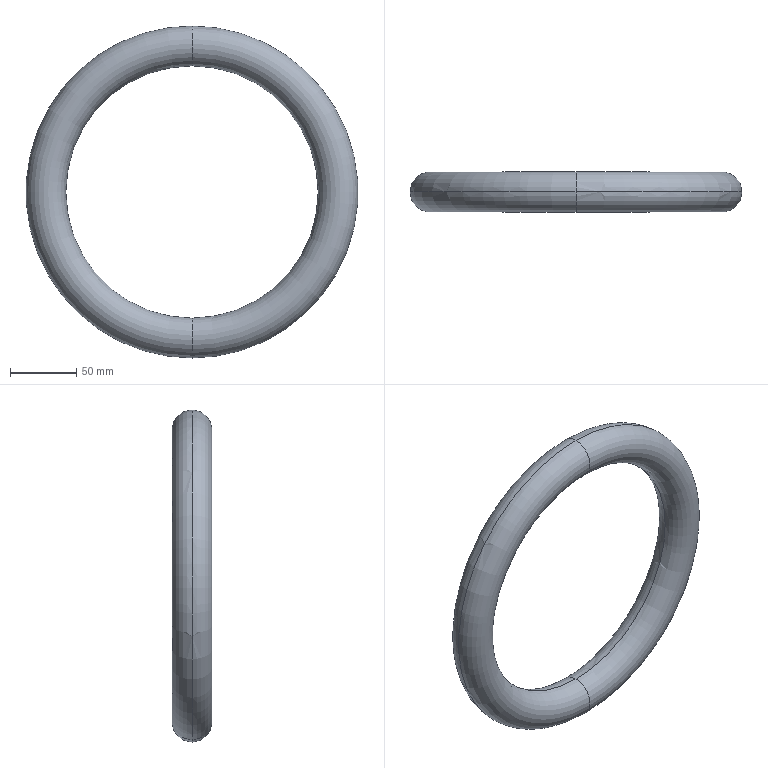Part | SolidWorks | features RefAxis 1, Revolution 1 | 1 solid | 4 faces | box 250 x 30 x 250 mm | volume 488545 mm3 | torus 4
STEP:
#1=CARTESIAN_POINT('',(0.,0.,125.));
#2=VERTEX_POINT('',#1);
#3=CARTESIAN_POINT('',(0.,0.,95.));
#4=VERTEX_POINT('',#3);
#5=CARTESIAN_POINT('',(0.,0.,110.));
#6=DIRECTION('',(1.,0.,0.));
#7=DIRECTION('',(0.,0.,-1.));
#8=AXIS2_PLACEMENT_3D('',#5,#6,#7);
#9=CIRCLE('',#8,15.);
#10=EDGE_CURVE('',#2,#4,#9,.T.);
#11=ORIENTED_EDGE('',*,*,#10,.F.);
#12=CARTESIAN_POINT('',(0.,0.,-125.));
#13=VERTEX_POINT('',#12);
#14=CARTESIAN_POINT('',(0.,0.,0.));
#15=DIRECTION('',(0.,-1.,0.));
#16=DIRECTION('',(0.,0.,-1.));
#17=AXIS2_PLACEMENT_3D('',#14,#15,#16);
#18=CIRCLE('',#17,125.);
#19=EDGE_CURVE('',#2,#13,#18,.T.);
#20=ORIENTED_EDGE('',*,*,#19,.T.);
#21=CARTESIAN_POINT('',(0.,0.,-95.));
#22=VERTEX_POINT('',#21);
#23=CARTESIAN_POINT('',(0.,0.,-110.));
#24=DIRECTION('',(-1.,0.,0.));
#25=DIRECTION('',(0.,0.,1.));
#26=AXIS2_PLACEMENT_3D('',#23,#24,#25);
#27=CIRCLE('',#26,15.);
#28=EDGE_CURVE('',#13,#22,#27,.T.);
#29=ORIENTED_EDGE('',*,*,#28,.T.);
#30=CARTESIAN_POINT('',(0.,0.,0.));
#31=DIRECTION('',(0.,-1.,0.));
#32=DIRECTION('',(0.,0.,-1.));
#33=AXIS2_PLACEMENT_3D('',#30,#31,#32);
#34=CIRCLE('',#33,95.);
#35=EDGE_CURVE('',#4,#22,#34,.T.);
#36=ORIENTED_EDGE('',*,*,#35,.F.);
#37=EDGE_LOOP('',(#11,#20,#29,#36));
#38=FACE_OUTER_BOUND('',#37,.T.);
#39=CARTESIAN_POINT('',(0.,0.,0.));
#40=DIRECTION('',(0.,-1.,0.));
#41=DIRECTION('',(0.,0.,-1.));
#42=AXIS2_PLACEMENT_3D('',#39,#40,#41);
#43=TOROIDAL_SURFACE('',#42,110.,15.);
#44=ADVANCED_FACE('',(#38),#43,.T.);
#45=ORIENTED_EDGE('',*,*,#28,.F.);
#46=CARTESIAN_POINT('',(0.,0.,0.));
#47=DIRECTION('',(0.,-1.,0.));
#48=DIRECTION('',(0.,0.,-1.));
#49=AXIS2_PLACEMENT_3D('',#46,#47,#48);
#50=CIRCLE('',#49,125.);
#51=EDGE_CURVE('',#13,#2,#50,.T.);
#52=ORIENTED_EDGE('',*,*,#51,.T.);
#53=ORIENTED_EDGE('',*,*,#10,.T.);
#54=CARTESIAN_POINT('',(0.,0.,0.));
#55=DIRECTION('',(0.,-1.,0.));
#56=DIRECTION('',(0.,0.,-1.));
#57=AXIS2_PLACEMENT_3D('',#54,#55,#56);
#58=CIRCLE('',#57,95.);
#59=EDGE_CURVE('',#22,#4,#58,.T.);
#60=ORIENTED_EDGE('',*,*,#59,.F.);
#61=EDGE_LOOP('',(#45,#52,#53,#60));
#62=FACE_OUTER_BOUND('',#61,.T.);
#63=CARTESIAN_POINT('',(0.,0.,0.));
#64=DIRECTION('',(0.,-1.,0.));
#65=DIRECTION('',(0.,0.,-1.));
#66=AXIS2_PLACEMENT_3D('',#63,#64,#65);
#67=TOROIDAL_SURFACE('',#66,110.,15.);
#68=ADVANCED_FACE('',(#62),#67,.T.);
#69=ORIENTED_EDGE('',*,*,#51,.F.);
#70=CARTESIAN_POINT('',(0.,0.,-110.));
#71=DIRECTION('',(-1.,0.,0.));
#72=DIRECTION('',(0.,0.,1.));
#73=AXIS2_PLACEMENT_3D('',#70,#71,#72);
#74=CIRCLE('',#73,15.);
#75=EDGE_CURVE('',#22,#13,#74,.T.);
#76=ORIENTED_EDGE('',*,*,#75,.F.);
#77=ORIENTED_EDGE('',*,*,#59,.T.);
#78=CARTESIAN_POINT('',(0.,0.,110.));
#79=DIRECTION('',(1.,0.,0.));
#80=DIRECTION('',(0.,0.,-1.));
#81=AXIS2_PLACEMENT_3D('',#78,#79,#80);
#82=CIRCLE('',#81,15.);
#83=EDGE_CURVE('',#4,#2,#82,.T.);
#84=ORIENTED_EDGE('',*,*,#83,.T.);
#85=EDGE_LOOP('',(#69,#76,#77,#84));
#86=FACE_OUTER_BOUND('',#85,.T.);
#87=CARTESIAN_POINT('',(0.,0.,0.));
#88=DIRECTION('',(0.,-1.,0.));
#89=DIRECTION('',(0.,0.,-1.));
#90=AXIS2_PLACEMENT_3D('',#87,#88,#89);
#91=TOROIDAL_SURFACE('',#90,110.,15.);
#92=ADVANCED_FACE('',(#86),#91,.T.);
#93=ORIENTED_EDGE('',*,*,#19,.F.);
#94=ORIENTED_EDGE('',*,*,#83,.F.);
#95=ORIENTED_EDGE('',*,*,#35,.T.);
#96=ORIENTED_EDGE('',*,*,#75,.T.);
#97=EDGE_LOOP('',(#93,#94,#95,#96));
#98=FACE_OUTER_BOUND('',#97,.T.);
#99=CARTESIAN_POINT('',(0.,0.,0.));
#100=DIRECTION('',(0.,-1.,0.));
#101=DIRECTION('',(0.,0.,-1.));
#102=AXIS2_PLACEMENT_3D('',#99,#100,#101);
#103=TOROIDAL_SURFACE('',#102,110.,15.);
#104=ADVANCED_FACE('',(#98),#103,.T.);
#105=CLOSED_SHELL('',(#44,#68,#92,#104));
#106=MANIFOLD_SOLID_BREP('',#105);
#107=CARTESIAN_POINT('',(0.,0.,0.));
#108=DIRECTION('',(0.,0.,1.));
#109=DIRECTION('',(1.,0.,0.));
#110=AXIS2_PLACEMENT_3D('',#107,#108,#109);
#111=(LENGTH_UNIT()NAMED_UNIT(*)SI_UNIT(.MILLI.,.METRE.));
#112=UNCERTAINTY_MEASURE_WITH_UNIT(LENGTH_MEASURE(0.00001),#111,'','');
#113=(NAMED_UNIT(*)PLANE_ANGLE_UNIT()SI_UNIT($,.RADIAN.));
#114=(NAMED_UNIT(*)SI_UNIT($,.STERADIAN.)SOLID_ANGLE_UNIT());
#115=(GEOMETRIC_REPRESENTATION_CONTEXT(3)GLOBAL_UNCERTAINTY_ASSIGNED_CONTEXT((#112))GLOBAL_UNIT_ASSIGNED_CONTEXT((#111,#113,#114))REPRESENTATION_CONTEXT('',''));
#116=ADVANCED_BREP_SHAPE_REPRESENTATION('',(#106,#110),#115);